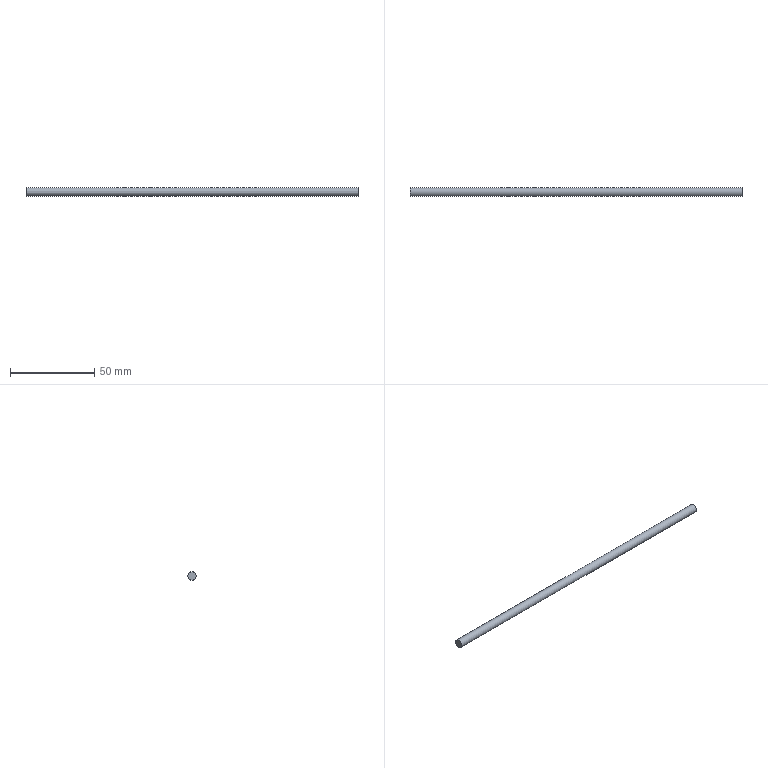Part | NX | features solid 2 | 1 solid | 3 faces | box 197 x 5 x 5 mm | volume 3868 mm3 | plane 2 | cylinder 1 | commonest cylinder face diameters 5 x1
STEP:
#1=CARTESIAN_POINT('',(-540.,-377.5,-432.5));
#2=VERTEX_POINT('',#1);
#3=CARTESIAN_POINT('',(-540.,-377.5,-430.));
#4=DIRECTION('',(1.,0.,0.));
#5=DIRECTION('',(0.,0.,-1.));
#6=AXIS2_PLACEMENT_3D('',#3,#4,#5);
#7=CIRCLE('',#6,2.5);
#8=EDGE_CURVE('',#2,#2,#7,.T.);
#9=ORIENTED_EDGE('',*,*,#8,.F.);
#10=EDGE_LOOP('',(#9));
#11=FACE_BOUND('',#10,.T.);
#12=CARTESIAN_POINT('',(-737.,-377.5,-432.5));
#13=VERTEX_POINT('',#12);
#14=CARTESIAN_POINT('',(-737.,-377.5,-430.));
#15=DIRECTION('',(1.,0.,0.));
#16=DIRECTION('',(0.,0.,-1.));
#17=AXIS2_PLACEMENT_3D('',#14,#15,#16);
#18=CIRCLE('',#17,2.5);
#19=EDGE_CURVE('',#13,#13,#18,.T.);
#20=ORIENTED_EDGE('',*,*,#19,.T.);
#21=EDGE_LOOP('',(#20));
#22=FACE_BOUND('',#21,.T.);
#23=CARTESIAN_POINT('',(-527.,-377.5,-430.));
#24=DIRECTION('',(-1.,0.,0.));
#25=DIRECTION('',(0.,0.,-1.));
#26=AXIS2_PLACEMENT_3D('',#23,#24,#25);
#27=CYLINDRICAL_SURFACE('',#26,2.5);
#28=ADVANCED_FACE('',(#11,#22),#27,.T.);
#29=ORIENTED_EDGE('',*,*,#8,.T.);
#30=EDGE_LOOP('',(#29));
#31=FACE_BOUND('',#30,.T.);
#32=CARTESIAN_POINT('',(-540.,80.624,-320.));
#33=DIRECTION('',(-1.,0.,0.));
#34=DIRECTION('',(0.,0.,-1.));
#35=AXIS2_PLACEMENT_3D('',#32,#33,#34);
#36=PLANE('',#35);
#37=ADVANCED_FACE('',(#31),#36,.F.);
#38=ORIENTED_EDGE('',*,*,#19,.F.);
#39=EDGE_LOOP('',(#38));
#40=FACE_BOUND('',#39,.T.);
#41=CARTESIAN_POINT('',(-737.,-377.5,-430.));
#42=DIRECTION('',(1.,0.,0.));
#43=DIRECTION('',(0.,0.,1.));
#44=AXIS2_PLACEMENT_3D('',#41,#42,#43);
#45=PLANE('',#44);
#46=ADVANCED_FACE('',(#40),#45,.F.);
#47=CLOSED_SHELL('',(#28,#37,#46));
#48=MANIFOLD_SOLID_BREP('',#47);
#49=(LENGTH_UNIT()NAMED_UNIT(*)SI_UNIT(.MILLI.,.METRE.));
#50=UNCERTAINTY_MEASURE_WITH_UNIT(LENGTH_MEASURE(0.00001),#49,'','');
#51=(NAMED_UNIT(*)PLANE_ANGLE_UNIT()SI_UNIT($,.RADIAN.));
#52=(NAMED_UNIT(*)SI_UNIT($,.STERADIAN.)SOLID_ANGLE_UNIT());
#53=(GEOMETRIC_REPRESENTATION_CONTEXT(3)GLOBAL_UNCERTAINTY_ASSIGNED_CONTEXT((#50))GLOBAL_UNIT_ASSIGNED_CONTEXT((#49,#51,#52))REPRESENTATION_CONTEXT('',''));
#54=ADVANCED_BREP_SHAPE_REPRESENTATION('',(#48),#53);